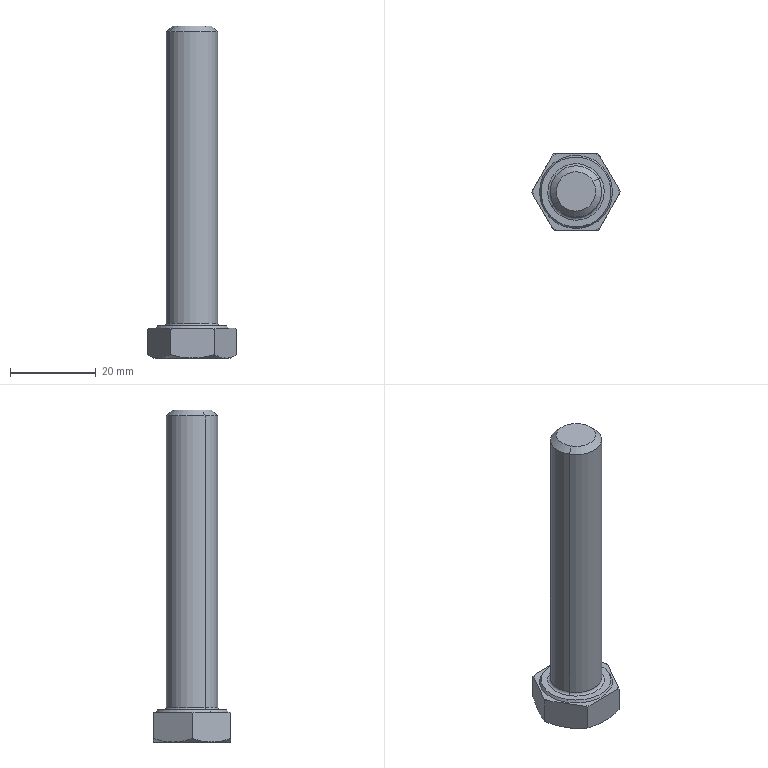Part | STEP file | BFACE2-29 | 1 solid | 30 faces | box 20.784 x 18.078 x 77.5 mm | volume 9947 mm3 | cone 16 | plane 10 | cylinder 2 | torus 2 | commonest cylinder face diameters 12 x2
STEP:
#1=CARTESIAN_POINT('',(-683.565,-263.234,3084.1));
#2=VERTEX_POINT('',#1);
#3=CARTESIAN_POINT('',(-693.912,-269.312,3084.1));
#4=VERTEX_POINT('',#3);
#5=CARTESIAN_POINT('',(-688.738,-266.273,3084.1));
#6=DIRECTION('',(0.,0.,-1.));
#7=DIRECTION('',(0.8622,0.5065,0.));
#8=AXIS2_PLACEMENT_3D('',#5,#6,#7);
#9=CIRCLE('',#8,6.);
#10=EDGE_CURVE('',#2,#4,#9,.T.);
#11=ORIENTED_EDGE('',*,*,#10,.F.);
#12=CARTESIAN_POINT('',(-683.565,-263.234,3152.1));
#13=VERTEX_POINT('',#12);
#14=CARTESIAN_POINT('',(-683.565,-263.234,3076.));
#15=DIRECTION('',(0.,0.,-1.));
#16=VECTOR('',#15,1000.);
#17=LINE('',#14,#16);
#18=EDGE_CURVE('',#13,#2,#17,.T.);
#19=ORIENTED_EDGE('',*,*,#18,.F.);
#20=CARTESIAN_POINT('',(-693.912,-269.312,3152.1));
#21=VERTEX_POINT('',#20);
#22=CARTESIAN_POINT('',(-688.738,-266.273,3152.1));
#23=DIRECTION('',(0.,0.,-1.));
#24=DIRECTION('',(-0.8622,-0.5065,0.));
#25=AXIS2_PLACEMENT_3D('',#22,#23,#24);
#26=CIRCLE('',#25,6.);
#27=EDGE_CURVE('',#13,#21,#26,.T.);
#28=ORIENTED_EDGE('',*,*,#27,.T.);
#29=CARTESIAN_POINT('',(-693.912,-269.312,3076.));
#30=DIRECTION('',(0.,0.,-1.));
#31=VECTOR('',#30,1000.);
#32=LINE('',#29,#31);
#33=EDGE_CURVE('',#21,#4,#32,.T.);
#34=ORIENTED_EDGE('',*,*,#33,.T.);
#35=EDGE_LOOP('',(#11,#19,#28,#34));
#36=FACE_OUTER_BOUND('',#35,.T.);
#37=CARTESIAN_POINT('',(-688.738,-266.273,3076.));
#38=DIRECTION('',(0.,0.,1.));
#39=DIRECTION('',(0.8622,0.5065,0.));
#40=AXIS2_PLACEMENT_3D('',#37,#38,#39);
#41=CYLINDRICAL_SURFACE('',#40,6.);
#42=ADVANCED_FACE('',(#36),#41,.T.);
#43=CARTESIAN_POINT('',(-692.705,-268.603,3153.5));
#44=VERTEX_POINT('',#43);
#45=CARTESIAN_POINT('',(-684.772,-263.943,3153.5));
#46=VERTEX_POINT('',#45);
#47=CARTESIAN_POINT('',(-688.738,-266.273,3153.5));
#48=DIRECTION('',(0.,0.,1.));
#49=DIRECTION('',(-0.8622,-0.5065,0.));
#50=AXIS2_PLACEMENT_3D('',#47,#48,#49);
#51=CIRCLE('',#50,4.6);
#52=EDGE_CURVE('',#44,#46,#51,.T.);
#53=ORIENTED_EDGE('',*,*,#52,.F.);
#54=CARTESIAN_POINT('',(-692.705,-268.603,3153.5));
#55=DIRECTION('',(-0.6097,-0.3582,-0.7071));
#56=VECTOR('',#55,1000.);
#57=LINE('',#54,#56);
#58=EDGE_CURVE('',#44,#21,#57,.T.);
#59=ORIENTED_EDGE('',*,*,#58,.T.);
#60=ORIENTED_EDGE('',*,*,#27,.F.);
#61=CARTESIAN_POINT('',(-684.772,-263.943,3153.5));
#62=DIRECTION('',(0.6097,0.3582,-0.7071));
#63=VECTOR('',#62,1000.);
#64=LINE('',#61,#63);
#65=EDGE_CURVE('',#46,#13,#64,.T.);
#66=ORIENTED_EDGE('',*,*,#65,.F.);
#67=EDGE_LOOP('',(#53,#59,#60,#66));
#68=FACE_OUTER_BOUND('',#67,.T.);
#69=CARTESIAN_POINT('',(-688.738,-266.273,3153.5));
#70=DIRECTION('',(0.,0.,-1.));
#71=DIRECTION('',(-0.8622,-0.5065,0.));
#72=AXIS2_PLACEMENT_3D('',#69,#70,#71);
#73=CONICAL_SURFACE('',#72,4.6,0.7854);
#74=ADVANCED_FACE('',(#68),#73,.T.);
#75=CARTESIAN_POINT('',(-694.429,-269.616,3083.5));
#76=VERTEX_POINT('',#75);
#77=CARTESIAN_POINT('',(-683.048,-262.93,3083.5));
#78=VERTEX_POINT('',#77);
#79=CARTESIAN_POINT('',(-688.738,-266.273,3083.5));
#80=DIRECTION('',(0.,0.,-1.));
#81=DIRECTION('',(0.8622,0.5065,0.));
#82=AXIS2_PLACEMENT_3D('',#79,#80,#81);
#83=CIRCLE('',#82,6.6);
#84=EDGE_CURVE('',#76,#78,#83,.T.);
#85=ORIENTED_EDGE('',*,*,#84,.F.);
#86=CARTESIAN_POINT('',(-694.429,-269.616,3084.1));
#87=DIRECTION('',(0.5065,-0.8622,0.));
#88=DIRECTION('',(0.8622,0.5065,0.));
#89=AXIS2_PLACEMENT_3D('',#86,#87,#88);
#90=CIRCLE('',#89,0.6);
#91=EDGE_CURVE('',#76,#4,#90,.T.);
#92=ORIENTED_EDGE('',*,*,#91,.T.);
#93=CARTESIAN_POINT('',(-688.738,-266.273,3084.1));
#94=DIRECTION('',(0.,0.,-1.));
#95=DIRECTION('',(0.8622,0.5065,0.));
#96=AXIS2_PLACEMENT_3D('',#93,#94,#95);
#97=CIRCLE('',#96,6.);
#98=EDGE_CURVE('',#4,#2,#97,.T.);
#99=ORIENTED_EDGE('',*,*,#98,.T.);
#100=CARTESIAN_POINT('',(-683.048,-262.93,3084.1));
#101=DIRECTION('',(-0.5065,0.8622,0.));
#102=DIRECTION('',(-0.8622,-0.5065,0.));
#103=AXIS2_PLACEMENT_3D('',#100,#101,#102);
#104=CIRCLE('',#103,0.6);
#105=EDGE_CURVE('',#78,#2,#104,.T.);
#106=ORIENTED_EDGE('',*,*,#105,.F.);
#107=EDGE_LOOP('',(#85,#92,#99,#106));
#108=FACE_OUTER_BOUND('',#107,.T.);
#109=CARTESIAN_POINT('',(-688.738,-266.273,3084.1));
#110=DIRECTION('',(0.,0.,-1.));
#111=DIRECTION('',(-0.8622,-0.5065,0.));
#112=AXIS2_PLACEMENT_3D('',#109,#110,#111);
#113=TOROIDAL_SURFACE('',#112,6.6,0.6);
#114=ADVANCED_FACE('',(#108),#113,.F.);
#115=CARTESIAN_POINT('',(-681.688,-262.131,3083.5));
#116=VERTEX_POINT('',#115);
#117=CARTESIAN_POINT('',(-695.789,-270.415,3083.5));
#118=VERTEX_POINT('',#117);
#119=CARTESIAN_POINT('',(-688.738,-266.273,3083.5));
#120=DIRECTION('',(0.,0.,-1.));
#121=DIRECTION('',(0.8622,0.5065,0.));
#122=AXIS2_PLACEMENT_3D('',#119,#120,#121);
#123=CIRCLE('',#122,8.177);
#124=EDGE_CURVE('',#116,#118,#123,.T.);
#125=ORIENTED_EDGE('',*,*,#124,.T.);
#126=CARTESIAN_POINT('',(-696.088,-270.59,3082.9));
#127=VERTEX_POINT('',#126);
#128=CARTESIAN_POINT('',(-696.088,-270.59,3082.9));
#129=DIRECTION('',(-0.4311,-0.2533,-0.866));
#130=VECTOR('',#129,1000.);
#131=LINE('',#128,#130);
#132=EDGE_CURVE('',#118,#127,#131,.T.);
#133=ORIENTED_EDGE('',*,*,#132,.T.);
#134=CARTESIAN_POINT('',(-681.389,-261.956,3082.9));
#135=VERTEX_POINT('',#134);
#136=CARTESIAN_POINT('',(-688.738,-266.273,3082.9));
#137=DIRECTION('',(0.,0.,-1.));
#138=DIRECTION('',(0.8622,0.5065,0.));
#139=AXIS2_PLACEMENT_3D('',#136,#137,#138);
#140=CIRCLE('',#139,8.524);
#141=EDGE_CURVE('',#135,#127,#140,.T.);
#142=ORIENTED_EDGE('',*,*,#141,.F.);
#143=CARTESIAN_POINT('',(-681.389,-261.956,3082.9));
#144=DIRECTION('',(0.4311,0.2533,-0.866));
#145=VECTOR('',#144,1000.);
#146=LINE('',#143,#145);
#147=EDGE_CURVE('',#116,#135,#146,.T.);
#148=ORIENTED_EDGE('',*,*,#147,.F.);
#149=EDGE_LOOP('',(#125,#133,#142,#148));
#150=FACE_OUTER_BOUND('',#149,.T.);
#151=CARTESIAN_POINT('',(-688.738,-266.273,3082.9));
#152=DIRECTION('',(0.,0.,-1.));
#153=DIRECTION('',(-0.8622,-0.5065,0.));
#154=AXIS2_PLACEMENT_3D('',#151,#152,#153);
#155=CONICAL_SURFACE('',#154,8.524,0.5236);
#156=ADVANCED_FACE('',(#150),#155,.T.);
#157=ORIENTED_EDGE('',*,*,#124,.F.);
#158=CARTESIAN_POINT('',(-688.738,-266.273,3083.5));
#159=DIRECTION('',(0.,0.,-1.));
#160=DIRECTION('',(0.8622,0.5065,0.));
#161=AXIS2_PLACEMENT_3D('',#158,#159,#160);
#162=CIRCLE('',#161,8.177);
#163=EDGE_CURVE('',#118,#116,#162,.T.);
#164=ORIENTED_EDGE('',*,*,#163,.F.);
#165=EDGE_LOOP('',(#157,#164));
#166=FACE_OUTER_BOUND('',#165,.T.);
#167=CARTESIAN_POINT('',(-688.738,-266.273,3083.5));
#168=DIRECTION('',(0.,0.,-1.));
#169=DIRECTION('',(0.8622,0.5065,0.));
#170=AXIS2_PLACEMENT_3D('',#167,#168,#169);
#171=CIRCLE('',#170,6.6);
#172=EDGE_CURVE('',#78,#76,#171,.T.);
#173=ORIENTED_EDGE('',*,*,#172,.T.);
#174=ORIENTED_EDGE('',*,*,#84,.T.);
#175=EDGE_LOOP('',(#173,#174));
#176=FACE_BOUND('',#175,.T.);
#177=CARTESIAN_POINT('',(-704.258,-275.39,3083.5));
#178=DIRECTION('',(0.,0.,1.));
#179=DIRECTION('',(0.8622,0.5065,0.));
#180=AXIS2_PLACEMENT_3D('',#177,#178,#179);
#181=PLANE('',#180);
#182=ADVANCED_FACE('',(#166,#176),#181,.T.);
#183=CARTESIAN_POINT('',(-693.118,-275.306,3082.9));
#184=VERTEX_POINT('',#183);
#185=CARTESIAN_POINT('',(-684.222,-275.239,3082.9));
#186=VERTEX_POINT('',#185);
#187=CARTESIAN_POINT('',(-693.866,-275.312,3082.9));
#188=DIRECTION('',(1.,0.007537,0.));
#189=VECTOR('',#188,1000.);
#190=LINE('',#187,#189);
#191=EDGE_CURVE('',#184,#186,#190,.T.);
#192=ORIENTED_EDGE('',*,*,#191,.F.);
#193=CARTESIAN_POINT('',(-693.866,-275.312,3082.696));
#194=VERTEX_POINT('',#193);
#195=CARTESIAN_POINT('',(-693.866,-275.312,3082.696));
#196=CARTESIAN_POINT('',(-693.618,-275.31,3082.768));
#197=CARTESIAN_POINT('',(-693.368,-275.308,3082.836));
#198=CARTESIAN_POINT('',(-693.118,-275.306,3082.9));
#199=B_SPLINE_CURVE_WITH_KNOTS('',3,(#195,#196,#197,#198),.UNSPECIFIED.,.F.,.F.,(4,4),(0.,1.),.UNSPECIFIED.);
#200=EDGE_CURVE('',#194,#184,#199,.T.);
#201=ORIENTED_EDGE('',*,*,#200,.F.);
#202=CARTESIAN_POINT('',(-693.866,-275.312,3076.804));
#203=VERTEX_POINT('',#202);
#204=CARTESIAN_POINT('',(-693.866,-275.312,3083.5));
#205=DIRECTION('',(0.,0.,-1.));
#206=VECTOR('',#205,1000.);
#207=LINE('',#204,#206);
#208=EDGE_CURVE('',#194,#203,#207,.T.);
#209=ORIENTED_EDGE('',*,*,#208,.T.);
#210=CARTESIAN_POINT('',(-688.67,-275.273,3076.));
#211=VERTEX_POINT('',#210);
#212=CARTESIAN_POINT('',(-688.67,-275.273,3076.));
#213=CARTESIAN_POINT('',(-689.557,-275.28,3076.));
#214=CARTESIAN_POINT('',(-690.432,-275.286,3076.077));
#215=CARTESIAN_POINT('',(-692.162,-275.299,3076.357));
#216=CARTESIAN_POINT('',(-693.018,-275.306,3076.559));
#217=CARTESIAN_POINT('',(-693.866,-275.312,3076.804));
#218=B_SPLINE_CURVE_WITH_KNOTS('',3,(#212,#213,#214,#215,#216,#217),.UNSPECIFIED.,.F.,.F.,(4,2,4),(0.,0.002629,0.005258),.UNSPECIFIED.);
#219=EDGE_CURVE('',#211,#203,#218,.T.);
#220=ORIENTED_EDGE('',*,*,#219,.F.);
#221=CARTESIAN_POINT('',(-683.474,-275.234,3076.804));
#222=VERTEX_POINT('',#221);
#223=CARTESIAN_POINT('',(-683.474,-275.234,3076.804));
#224=CARTESIAN_POINT('',(-684.323,-275.24,3076.559));
#225=CARTESIAN_POINT('',(-685.179,-275.247,3076.357));
#226=CARTESIAN_POINT('',(-686.909,-275.26,3076.077));
#227=CARTESIAN_POINT('',(-687.784,-275.266,3076.));
#228=CARTESIAN_POINT('',(-688.67,-275.273,3076.));
#229=B_SPLINE_CURVE_WITH_KNOTS('',3,(#223,#224,#225,#226,#227,#228),.UNSPECIFIED.,.F.,.F.,(4,2,4),(0.,0.002629,0.005258),.UNSPECIFIED.);
#230=EDGE_CURVE('',#222,#211,#229,.T.);
#231=ORIENTED_EDGE('',*,*,#230,.F.);
#232=CARTESIAN_POINT('',(-683.474,-275.234,3082.696));
#233=VERTEX_POINT('',#232);
#234=CARTESIAN_POINT('',(-683.474,-275.234,3083.5));
#235=DIRECTION('',(0.,0.,-1.));
#236=VECTOR('',#235,1000.);
#237=LINE('',#234,#236);
#238=EDGE_CURVE('',#233,#222,#237,.T.);
#239=ORIENTED_EDGE('',*,*,#238,.F.);
#240=CARTESIAN_POINT('',(-684.222,-275.239,3082.9));
#241=CARTESIAN_POINT('',(-683.972,-275.237,3082.836));
#242=CARTESIAN_POINT('',(-683.723,-275.236,3082.768));
#243=CARTESIAN_POINT('',(-683.474,-275.234,3082.696));
#244=B_SPLINE_CURVE_WITH_KNOTS('',3,(#240,#241,#242,#243),.UNSPECIFIED.,.F.,.F.,(4,4),(0.,1.),.UNSPECIFIED.);
#245=EDGE_CURVE('',#186,#233,#244,.T.);
#246=ORIENTED_EDGE('',*,*,#245,.F.);
#247=EDGE_LOOP('',(#192,#201,#209,#220,#231,#239,#246));
#248=FACE_OUTER_BOUND('',#247,.T.);
#249=CARTESIAN_POINT('',(-693.866,-275.312,3083.5));
#250=DIRECTION('',(-0.007537,1.,0.));
#251=DIRECTION('',(1.,0.007537,0.));
#252=AXIS2_PLACEMENT_3D('',#249,#250,#251);
#253=PLANE('',#252);
#254=ADVANCED_FACE('',(#248),#253,.F.);
#255=CARTESIAN_POINT('',(-683.105,-274.583,3082.9));
#256=VERTEX_POINT('',#255);
#257=CARTESIAN_POINT('',(-678.715,-266.845,3082.9));
#258=VERTEX_POINT('',#257);
#259=CARTESIAN_POINT('',(-683.474,-275.234,3082.9));
#260=DIRECTION('',(0.4935,0.8698,0.));
#261=VECTOR('',#260,1000.);
#262=LINE('',#259,#261);
#263=EDGE_CURVE('',#256,#258,#262,.T.);
#264=ORIENTED_EDGE('',*,*,#263,.F.);
#265=CARTESIAN_POINT('',(-683.474,-275.234,3082.696));
#266=CARTESIAN_POINT('',(-683.352,-275.017,3082.768));
#267=CARTESIAN_POINT('',(-683.229,-274.8,3082.836));
#268=CARTESIAN_POINT('',(-683.105,-274.583,3082.9));
#269=B_SPLINE_CURVE_WITH_KNOTS('',3,(#265,#266,#267,#268),.UNSPECIFIED.,.F.,.F.,(4,4),(0.,1.),.UNSPECIFIED.);
#270=EDGE_CURVE('',#233,#256,#269,.T.);
#271=ORIENTED_EDGE('',*,*,#270,.F.);
#272=ORIENTED_EDGE('',*,*,#238,.T.);
#273=CARTESIAN_POINT('',(-680.91,-270.714,3076.));
#274=VERTEX_POINT('',#273);
#275=CARTESIAN_POINT('',(-680.91,-270.714,3076.));
#276=CARTESIAN_POINT('',(-681.348,-271.486,3076.));
#277=CARTESIAN_POINT('',(-681.78,-272.246,3076.077));
#278=CARTESIAN_POINT('',(-682.633,-273.751,3076.357));
#279=CARTESIAN_POINT('',(-683.056,-274.495,3076.559));
#280=CARTESIAN_POINT('',(-683.474,-275.234,3076.804));
#281=B_SPLINE_CURVE_WITH_KNOTS('',3,(#275,#276,#277,#278,#279,#280),.UNSPECIFIED.,.F.,.F.,(4,2,4),(0.,0.002629,0.005258),.UNSPECIFIED.);
#282=EDGE_CURVE('',#274,#222,#281,.T.);
#283=ORIENTED_EDGE('',*,*,#282,.F.);
#284=CARTESIAN_POINT('',(-678.346,-266.195,3076.804));
#285=VERTEX_POINT('',#284);
#286=CARTESIAN_POINT('',(-678.346,-266.195,3076.804));
#287=CARTESIAN_POINT('',(-678.765,-266.933,3076.559));
#288=CARTESIAN_POINT('',(-679.187,-267.677,3076.357));
#289=CARTESIAN_POINT('',(-680.041,-269.182,3076.077));
#290=CARTESIAN_POINT('',(-680.473,-269.943,3076.));
#291=CARTESIAN_POINT('',(-680.91,-270.714,3076.));
#292=B_SPLINE_CURVE_WITH_KNOTS('',3,(#286,#287,#288,#289,#290,#291),.UNSPECIFIED.,.F.,.F.,(4,2,4),(0.,0.002629,0.005258),.UNSPECIFIED.);
#293=EDGE_CURVE('',#285,#274,#292,.T.);
#294=ORIENTED_EDGE('',*,*,#293,.F.);
#295=CARTESIAN_POINT('',(-678.346,-266.195,3082.696));
#296=VERTEX_POINT('',#295);
#297=CARTESIAN_POINT('',(-678.346,-266.195,3083.5));
#298=DIRECTION('',(0.,0.,-1.));
#299=VECTOR('',#298,1000.);
#300=LINE('',#297,#299);
#301=EDGE_CURVE('',#296,#285,#300,.T.);
#302=ORIENTED_EDGE('',*,*,#301,.F.);
#303=CARTESIAN_POINT('',(-678.715,-266.845,3082.9));
#304=CARTESIAN_POINT('',(-678.592,-266.628,3082.836));
#305=CARTESIAN_POINT('',(-678.469,-266.411,3082.768));
#306=CARTESIAN_POINT('',(-678.346,-266.195,3082.696));
#307=B_SPLINE_CURVE_WITH_KNOTS('',3,(#303,#304,#305,#306),.UNSPECIFIED.,.F.,.F.,(4,4),(0.,1.),.UNSPECIFIED.);
#308=EDGE_CURVE('',#258,#296,#307,.T.);
#309=ORIENTED_EDGE('',*,*,#308,.F.);
#310=EDGE_LOOP('',(#264,#271,#272,#283,#294,#302,#309));
#311=FACE_OUTER_BOUND('',#310,.T.);
#312=CARTESIAN_POINT('',(-683.474,-275.234,3083.5));
#313=DIRECTION('',(-0.8698,0.4935,0.));
#314=DIRECTION('',(0.4935,0.8698,0.));
#315=AXIS2_PLACEMENT_3D('',#312,#313,#314);
#316=PLANE('',#315);
#317=ADVANCED_FACE('',(#311),#316,.F.);
#318=CARTESIAN_POINT('',(-678.725,-265.55,3082.9));
#319=VERTEX_POINT('',#318);
#320=CARTESIAN_POINT('',(-683.231,-257.879,3082.9));
#321=VERTEX_POINT('',#320);
#322=CARTESIAN_POINT('',(-678.346,-266.195,3082.9));
#323=DIRECTION('',(-0.5065,0.8622,0.));
#324=VECTOR('',#323,1000.);
#325=LINE('',#322,#324);
#326=EDGE_CURVE('',#319,#321,#325,.T.);
#327=ORIENTED_EDGE('',*,*,#326,.F.);
#328=CARTESIAN_POINT('',(-678.346,-266.195,3082.696));
#329=CARTESIAN_POINT('',(-678.472,-265.981,3082.768));
#330=CARTESIAN_POINT('',(-678.598,-265.766,3082.836));
#331=CARTESIAN_POINT('',(-678.725,-265.55,3082.9));
#332=B_SPLINE_CURVE_WITH_KNOTS('',3,(#328,#329,#330,#331),.UNSPECIFIED.,.F.,.F.,(4,4),(0.,1.),.UNSPECIFIED.);
#333=EDGE_CURVE('',#296,#319,#332,.T.);
#334=ORIENTED_EDGE('',*,*,#333,.F.);
#335=ORIENTED_EDGE('',*,*,#301,.T.);
#336=CARTESIAN_POINT('',(-680.978,-261.715,3076.));
#337=VERTEX_POINT('',#336);
#338=CARTESIAN_POINT('',(-680.978,-261.715,3076.));
#339=CARTESIAN_POINT('',(-680.529,-262.479,3076.));
#340=CARTESIAN_POINT('',(-680.086,-263.233,3076.077));
#341=CARTESIAN_POINT('',(-679.21,-264.725,3076.357));
#342=CARTESIAN_POINT('',(-678.776,-265.463,3076.559));
#343=CARTESIAN_POINT('',(-678.346,-266.195,3076.804));
#344=B_SPLINE_CURVE_WITH_KNOTS('',3,(#338,#339,#340,#341,#342,#343),.UNSPECIFIED.,.F.,.F.,(4,2,4),(0.,0.002629,0.005258),.UNSPECIFIED.);
#345=EDGE_CURVE('',#337,#285,#344,.T.);
#346=ORIENTED_EDGE('',*,*,#345,.F.);
#347=CARTESIAN_POINT('',(-683.61,-257.234,3076.804));
#348=VERTEX_POINT('',#347);
#349=CARTESIAN_POINT('',(-683.61,-257.234,3076.804));
#350=CARTESIAN_POINT('',(-683.18,-257.966,3076.559));
#351=CARTESIAN_POINT('',(-682.747,-258.704,3076.357));
#352=CARTESIAN_POINT('',(-681.87,-260.196,3076.077));
#353=CARTESIAN_POINT('',(-681.427,-260.95,3076.));
#354=CARTESIAN_POINT('',(-680.978,-261.715,3076.));
#355=B_SPLINE_CURVE_WITH_KNOTS('',3,(#349,#350,#351,#352,#353,#354),.UNSPECIFIED.,.F.,.F.,(4,2,4),(0.,0.002629,0.005258),.UNSPECIFIED.);
#356=EDGE_CURVE('',#348,#337,#355,.T.);
#357=ORIENTED_EDGE('',*,*,#356,.F.);
#358=CARTESIAN_POINT('',(-683.61,-257.234,3082.696));
#359=VERTEX_POINT('',#358);
#360=CARTESIAN_POINT('',(-683.61,-257.234,3083.5));
#361=DIRECTION('',(0.,0.,-1.));
#362=VECTOR('',#361,1000.);
#363=LINE('',#360,#362);
#364=EDGE_CURVE('',#359,#348,#363,.T.);
#365=ORIENTED_EDGE('',*,*,#364,.F.);
#366=CARTESIAN_POINT('',(-683.231,-257.879,3082.9));
#367=CARTESIAN_POINT('',(-683.358,-257.663,3082.836));
#368=CARTESIAN_POINT('',(-683.485,-257.448,3082.768));
#369=CARTESIAN_POINT('',(-683.61,-257.234,3082.696));
#370=B_SPLINE_CURVE_WITH_KNOTS('',3,(#366,#367,#368,#369),.UNSPECIFIED.,.F.,.F.,(4,4),(0.,1.),.UNSPECIFIED.);
#371=EDGE_CURVE('',#321,#359,#370,.T.);
#372=ORIENTED_EDGE('',*,*,#371,.F.);
#373=EDGE_LOOP('',(#327,#334,#335,#346,#357,#365,#372));
#374=FACE_OUTER_BOUND('',#373,.T.);
#375=CARTESIAN_POINT('',(-678.346,-266.195,3083.5));
#376=DIRECTION('',(-0.8622,-0.5065,0.));
#377=DIRECTION('',(-0.5065,0.8622,0.));
#378=AXIS2_PLACEMENT_3D('',#375,#376,#377);
#379=PLANE('',#378);
#380=ADVANCED_FACE('',(#374),#379,.F.);
#381=CARTESIAN_POINT('',(-684.358,-257.24,3082.9));
#382=VERTEX_POINT('',#381);
#383=CARTESIAN_POINT('',(-693.254,-257.307,3082.9));
#384=VERTEX_POINT('',#383);
#385=CARTESIAN_POINT('',(-694.002,-257.313,3082.9));
#386=DIRECTION('',(-1.,-0.007537,0.));
#387=VECTOR('',#386,1000.);
#388=LINE('',#385,#387);
#389=EDGE_CURVE('',#382,#384,#388,.T.);
#390=ORIENTED_EDGE('',*,*,#389,.F.);
#391=CARTESIAN_POINT('',(-683.61,-257.234,3082.696));
#392=CARTESIAN_POINT('',(-683.859,-257.236,3082.768));
#393=CARTESIAN_POINT('',(-684.108,-257.238,3082.836));
#394=CARTESIAN_POINT('',(-684.358,-257.24,3082.9));
#395=B_SPLINE_CURVE_WITH_KNOTS('',3,(#391,#392,#393,#394),.UNSPECIFIED.,.F.,.F.,(4,4),(0.,1.),.UNSPECIFIED.);
#396=EDGE_CURVE('',#359,#382,#395,.T.);
#397=ORIENTED_EDGE('',*,*,#396,.F.);
#398=ORIENTED_EDGE('',*,*,#364,.T.);
#399=CARTESIAN_POINT('',(-688.806,-257.273,3076.));
#400=VERTEX_POINT('',#399);
#401=CARTESIAN_POINT('',(-688.806,-257.273,3076.));
#402=CARTESIAN_POINT('',(-687.919,-257.267,3076.));
#403=CARTESIAN_POINT('',(-687.045,-257.26,3076.077));
#404=CARTESIAN_POINT('',(-685.314,-257.247,3076.357));
#405=CARTESIAN_POINT('',(-684.459,-257.241,3076.559));
#406=CARTESIAN_POINT('',(-683.61,-257.234,3076.804));
#407=B_SPLINE_CURVE_WITH_KNOTS('',3,(#401,#402,#403,#404,#405,#406),.UNSPECIFIED.,.F.,.F.,(4,2,4),(0.,0.002629,0.005258),.UNSPECIFIED.);
#408=EDGE_CURVE('',#400,#348,#407,.T.);
#409=ORIENTED_EDGE('',*,*,#408,.F.);
#410=CARTESIAN_POINT('',(-694.002,-257.313,3076.804));
#411=VERTEX_POINT('',#410);
#412=CARTESIAN_POINT('',(-694.002,-257.313,3076.804));
#413=CARTESIAN_POINT('',(-693.153,-257.306,3076.559));
#414=CARTESIAN_POINT('',(-692.298,-257.3,3076.357));
#415=CARTESIAN_POINT('',(-690.568,-257.287,3076.077));
#416=CARTESIAN_POINT('',(-689.693,-257.28,3076.));
#417=CARTESIAN_POINT('',(-688.806,-257.273,3076.));
#418=B_SPLINE_CURVE_WITH_KNOTS('',3,(#412,#413,#414,#415,#416,#417),.UNSPECIFIED.,.F.,.F.,(4,2,4),(0.,0.002629,0.005258),.UNSPECIFIED.);
#419=EDGE_CURVE('',#411,#400,#418,.T.);
#420=ORIENTED_EDGE('',*,*,#419,.F.);
#421=CARTESIAN_POINT('',(-694.002,-257.313,3082.696));
#422=VERTEX_POINT('',#421);
#423=CARTESIAN_POINT('',(-694.002,-257.313,3083.5));
#424=DIRECTION('',(0.,0.,-1.));
#425=VECTOR('',#424,1000.);
#426=LINE('',#423,#425);
#427=EDGE_CURVE('',#422,#411,#426,.T.);
#428=ORIENTED_EDGE('',*,*,#427,.F.);
#429=CARTESIAN_POINT('',(-693.254,-257.307,3082.9));
#430=CARTESIAN_POINT('',(-693.504,-257.309,3082.836));
#431=CARTESIAN_POINT('',(-693.753,-257.311,3082.768));
#432=CARTESIAN_POINT('',(-694.002,-257.313,3082.696));
#433=B_SPLINE_CURVE_WITH_KNOTS('',3,(#429,#430,#431,#432),.UNSPECIFIED.,.F.,.F.,(4,4),(0.,1.),.UNSPECIFIED.);
#434=EDGE_CURVE('',#384,#422,#433,.T.);
#435=ORIENTED_EDGE('',*,*,#434,.F.);
#436=EDGE_LOOP('',(#390,#397,#398,#409,#420,#428,#435));
#437=FACE_OUTER_BOUND('',#436,.T.);
#438=CARTESIAN_POINT('',(-694.002,-257.313,3083.5));
#439=DIRECTION('',(0.007537,-1.,0.));
#440=DIRECTION('',(-1.,-0.007537,0.));
#441=AXIS2_PLACEMENT_3D('',#438,#439,#440);
#442=PLANE('',#441);
#443=ADVANCED_FACE('',(#437),#442,.F.);
#444=CARTESIAN_POINT('',(-694.371,-257.963,3082.9));
#445=VERTEX_POINT('',#444);
#446=CARTESIAN_POINT('',(-698.761,-265.701,3082.9));
#447=VERTEX_POINT('',#446);
#448=CARTESIAN_POINT('',(-699.13,-266.351,3082.9));
#449=DIRECTION('',(-0.4935,-0.8698,0.));
#450=VECTOR('',#449,1000.);
#451=LINE('',#448,#450);
#452=EDGE_CURVE('',#445,#447,#451,.T.);
#453=ORIENTED_EDGE('',*,*,#452,.F.);
#454=CARTESIAN_POINT('',(-694.002,-257.313,3082.696));
#455=CARTESIAN_POINT('',(-694.125,-257.529,3082.768));
#456=CARTESIAN_POINT('',(-694.248,-257.746,3082.836));
#457=CARTESIAN_POINT('',(-694.371,-257.963,3082.9));
#458=B_SPLINE_CURVE_WITH_KNOTS('',3,(#454,#455,#456,#457),.UNSPECIFIED.,.F.,.F.,(4,4),(0.,1.),.UNSPECIFIED.);
#459=EDGE_CURVE('',#422,#445,#458,.T.);
#460=ORIENTED_EDGE('',*,*,#459,.F.);
#461=ORIENTED_EDGE('',*,*,#427,.T.);
#462=CARTESIAN_POINT('',(-696.566,-261.832,3076.));
#463=VERTEX_POINT('',#462);
#464=CARTESIAN_POINT('',(-696.566,-261.832,3076.));
#465=CARTESIAN_POINT('',(-696.129,-261.061,3076.));
#466=CARTESIAN_POINT('',(-695.697,-260.3,3076.077));
#467=CARTESIAN_POINT('',(-694.843,-258.795,3076.357));
#468=CARTESIAN_POINT('',(-694.421,-258.051,3076.559));
#469=CARTESIAN_POINT('',(-694.002,-257.313,3076.804));
#470=B_SPLINE_CURVE_WITH_KNOTS('',3,(#464,#465,#466,#467,#468,#469),.UNSPECIFIED.,.F.,.F.,(4,2,4),(0.,0.002629,0.005258),.UNSPECIFIED.);
#471=EDGE_CURVE('',#463,#411,#470,.T.);
#472=ORIENTED_EDGE('',*,*,#471,.F.);
#473=CARTESIAN_POINT('',(-699.13,-266.351,3076.804));
#474=VERTEX_POINT('',#473);
#475=CARTESIAN_POINT('',(-699.13,-266.351,3076.804));
#476=CARTESIAN_POINT('',(-698.711,-265.613,3076.559));
#477=CARTESIAN_POINT('',(-698.289,-264.869,3076.357));
#478=CARTESIAN_POINT('',(-697.435,-263.364,3076.077));
#479=CARTESIAN_POINT('',(-697.004,-262.603,3076.));
#480=CARTESIAN_POINT('',(-696.566,-261.832,3076.));
#481=B_SPLINE_CURVE_WITH_KNOTS('',3,(#475,#476,#477,#478,#479,#480),.UNSPECIFIED.,.F.,.F.,(4,2,4),(0.,0.002629,0.005258),.UNSPECIFIED.);
#482=EDGE_CURVE('',#474,#463,#481,.T.);
#483=ORIENTED_EDGE('',*,*,#482,.F.);
#484=CARTESIAN_POINT('',(-699.13,-266.351,3082.696));
#485=VERTEX_POINT('',#484);
#486=CARTESIAN_POINT('',(-699.13,-266.351,3083.5));
#487=DIRECTION('',(0.,0.,-1.));
#488=VECTOR('',#487,1000.);
#489=LINE('',#486,#488);
#490=EDGE_CURVE('',#485,#474,#489,.T.);
#491=ORIENTED_EDGE('',*,*,#490,.F.);
#492=CARTESIAN_POINT('',(-698.761,-265.701,3082.9));
#493=CARTESIAN_POINT('',(-698.885,-265.918,3082.836));
#494=CARTESIAN_POINT('',(-699.008,-266.135,3082.768));
#495=CARTESIAN_POINT('',(-699.13,-266.351,3082.696));
#496=B_SPLINE_CURVE_WITH_KNOTS('',3,(#492,#493,#494,#495),.UNSPECIFIED.,.F.,.F.,(4,4),(0.,1.),.UNSPECIFIED.);
#497=EDGE_CURVE('',#447,#485,#496,.T.);
#498=ORIENTED_EDGE('',*,*,#497,.F.);
#499=EDGE_LOOP('',(#453,#460,#461,#472,#483,#491,#498));
#500=FACE_OUTER_BOUND('',#499,.T.);
#501=CARTESIAN_POINT('',(-699.13,-266.351,3083.5));
#502=DIRECTION('',(0.8698,-0.4935,0.));
#503=DIRECTION('',(-0.4935,-0.8698,0.));
#504=AXIS2_PLACEMENT_3D('',#501,#502,#503);
#505=PLANE('',#504);
#506=ADVANCED_FACE('',(#500),#505,.F.);
#507=CARTESIAN_POINT('',(-698.751,-266.996,3082.9));
#508=VERTEX_POINT('',#507);
#509=CARTESIAN_POINT('',(-694.245,-274.667,3082.9));
#510=VERTEX_POINT('',#509);
#511=CARTESIAN_POINT('',(-693.866,-275.312,3082.9));
#512=DIRECTION('',(0.5065,-0.8622,0.));
#513=VECTOR('',#512,1000.);
#514=LINE('',#511,#513);
#515=EDGE_CURVE('',#508,#510,#514,.T.);
#516=ORIENTED_EDGE('',*,*,#515,.F.);
#517=CARTESIAN_POINT('',(-699.13,-266.351,3082.696));
#518=CARTESIAN_POINT('',(-699.005,-266.565,3082.768));
#519=CARTESIAN_POINT('',(-698.878,-266.78,3082.836));
#520=CARTESIAN_POINT('',(-698.751,-266.996,3082.9));
#521=B_SPLINE_CURVE_WITH_KNOTS('',3,(#517,#518,#519,#520),.UNSPECIFIED.,.F.,.F.,(4,4),(0.,1.),.UNSPECIFIED.);
#522=EDGE_CURVE('',#485,#508,#521,.T.);
#523=ORIENTED_EDGE('',*,*,#522,.F.);
#524=ORIENTED_EDGE('',*,*,#490,.T.);
#525=CARTESIAN_POINT('',(-696.498,-270.832,3076.));
#526=VERTEX_POINT('',#525);
#527=CARTESIAN_POINT('',(-696.498,-270.832,3076.));
#528=CARTESIAN_POINT('',(-696.948,-270.067,3076.));
#529=CARTESIAN_POINT('',(-697.391,-269.313,3076.077));
#530=CARTESIAN_POINT('',(-698.267,-267.821,3076.357));
#531=CARTESIAN_POINT('',(-698.7,-267.083,3076.559));
#532=CARTESIAN_POINT('',(-699.13,-266.351,3076.804));
#533=B_SPLINE_CURVE_WITH_KNOTS('',3,(#527,#528,#529,#530,#531,#532),.UNSPECIFIED.,.F.,.F.,(4,2,4),(0.,0.002629,0.005258),.UNSPECIFIED.);
#534=EDGE_CURVE('',#526,#474,#533,.T.);
#535=ORIENTED_EDGE('',*,*,#534,.F.);
#536=CARTESIAN_POINT('',(-693.866,-275.312,3076.804));
#537=CARTESIAN_POINT('',(-694.296,-274.58,3076.559));
#538=CARTESIAN_POINT('',(-694.73,-273.843,3076.357));
#539=CARTESIAN_POINT('',(-695.606,-272.351,3076.077));
#540=CARTESIAN_POINT('',(-696.049,-271.596,3076.));
#541=CARTESIAN_POINT('',(-696.498,-270.832,3076.));
#542=B_SPLINE_CURVE_WITH_KNOTS('',3,(#536,#537,#538,#539,#540,#541),.UNSPECIFIED.,.F.,.F.,(4,2,4),(0.,0.002629,0.005258),.UNSPECIFIED.);
#543=EDGE_CURVE('',#203,#526,#542,.T.);
#544=ORIENTED_EDGE('',*,*,#543,.F.);
#545=ORIENTED_EDGE('',*,*,#208,.F.);
#546=CARTESIAN_POINT('',(-694.245,-274.667,3082.9));
#547=CARTESIAN_POINT('',(-694.119,-274.883,3082.836));
#548=CARTESIAN_POINT('',(-693.992,-275.098,3082.768));
#549=CARTESIAN_POINT('',(-693.866,-275.312,3082.696));
#550=B_SPLINE_CURVE_WITH_KNOTS('',3,(#546,#547,#548,#549),.UNSPECIFIED.,.F.,.F.,(4,4),(0.,1.),.UNSPECIFIED.);
#551=EDGE_CURVE('',#510,#194,#550,.T.);
#552=ORIENTED_EDGE('',*,*,#551,.F.);
#553=EDGE_LOOP('',(#516,#523,#524,#535,#544,#545,#552));
#554=FACE_OUTER_BOUND('',#553,.T.);
#555=CARTESIAN_POINT('',(-693.866,-275.312,3083.5));
#556=DIRECTION('',(0.8622,0.5065,0.));
#557=DIRECTION('',(0.5065,-0.8622,0.));
#558=AXIS2_PLACEMENT_3D('',#555,#556,#557);
#559=PLANE('',#558);
#560=ADVANCED_FACE('',(#554),#559,.F.);
#561=ORIENTED_EDGE('',*,*,#522,.T.);
#562=CARTESIAN_POINT('',(-688.738,-266.273,3082.9));
#563=DIRECTION('',(0.,0.,-1.));
#564=DIRECTION('',(-0.8622,-0.5065,0.));
#565=AXIS2_PLACEMENT_3D('',#562,#563,#564);
#566=CIRCLE('',#565,10.039);
#567=EDGE_CURVE('',#508,#447,#566,.T.);
#568=ORIENTED_EDGE('',*,*,#567,.T.);
#569=ORIENTED_EDGE('',*,*,#497,.T.);
#570=EDGE_LOOP('',(#561,#568,#569));
#571=FACE_OUTER_BOUND('',#570,.T.);
#572=CARTESIAN_POINT('',(-688.738,-266.273,3079.809));
#573=DIRECTION('',(0.,0.,-1.));
#574=DIRECTION('',(-0.8622,-0.5065,0.));
#575=AXIS2_PLACEMENT_3D('',#572,#573,#574);
#576=CONICAL_SURFACE('',#575,15.392,1.047);
#577=ADVANCED_FACE('',(#571),#576,.T.);
#578=ORIENTED_EDGE('',*,*,#459,.T.);
#579=CARTESIAN_POINT('',(-688.738,-266.273,3082.9));
#580=DIRECTION('',(0.,0.,-1.));
#581=DIRECTION('',(-0.8622,-0.5065,0.));
#582=AXIS2_PLACEMENT_3D('',#579,#580,#581);
#583=CIRCLE('',#582,10.039);
#584=EDGE_CURVE('',#445,#384,#583,.T.);
#585=ORIENTED_EDGE('',*,*,#584,.T.);
#586=ORIENTED_EDGE('',*,*,#434,.T.);
#587=EDGE_LOOP('',(#578,#585,#586));
#588=FACE_OUTER_BOUND('',#587,.T.);
#589=CARTESIAN_POINT('',(-688.738,-266.273,3079.809));
#590=DIRECTION('',(0.,0.,-1.));
#591=DIRECTION('',(-0.8622,-0.5065,0.));
#592=AXIS2_PLACEMENT_3D('',#589,#590,#591);
#593=CONICAL_SURFACE('',#592,15.392,1.047);
#594=ADVANCED_FACE('',(#588),#593,.T.);
#595=ORIENTED_EDGE('',*,*,#396,.T.);
#596=CARTESIAN_POINT('',(-688.738,-266.273,3082.9));
#597=DIRECTION('',(0.,0.,-1.));
#598=DIRECTION('',(-0.8622,-0.5065,0.));
#599=AXIS2_PLACEMENT_3D('',#596,#597,#598);
#600=CIRCLE('',#599,10.039);
#601=EDGE_CURVE('',#382,#321,#600,.T.);
#602=ORIENTED_EDGE('',*,*,#601,.T.);
#603=ORIENTED_EDGE('',*,*,#371,.T.);
#604=EDGE_LOOP('',(#595,#602,#603));
#605=FACE_OUTER_BOUND('',#604,.T.);
#606=CARTESIAN_POINT('',(-688.738,-266.273,3079.809));
#607=DIRECTION('',(0.,0.,-1.));
#608=DIRECTION('',(-0.8622,-0.5065,0.));
#609=AXIS2_PLACEMENT_3D('',#606,#607,#608);
#610=CONICAL_SURFACE('',#609,15.392,1.047);
#611=ADVANCED_FACE('',(#605),#610,.T.);
#612=ORIENTED_EDGE('',*,*,#333,.T.);
#613=CARTESIAN_POINT('',(-688.738,-266.273,3082.9));
#614=DIRECTION('',(0.,0.,-1.));
#615=DIRECTION('',(-0.8622,-0.5065,0.));
#616=AXIS2_PLACEMENT_3D('',#613,#614,#615);
#617=CIRCLE('',#616,10.039);
#618=EDGE_CURVE('',#319,#258,#617,.T.);
#619=ORIENTED_EDGE('',*,*,#618,.T.);
#620=ORIENTED_EDGE('',*,*,#308,.T.);
#621=EDGE_LOOP('',(#612,#619,#620));
#622=FACE_OUTER_BOUND('',#621,.T.);
#623=CARTESIAN_POINT('',(-688.738,-266.273,3079.809));
#624=DIRECTION('',(0.,0.,-1.));
#625=DIRECTION('',(-0.8622,-0.5065,0.));
#626=AXIS2_PLACEMENT_3D('',#623,#624,#625);
#627=CONICAL_SURFACE('',#626,15.392,1.047);
#628=ADVANCED_FACE('',(#622),#627,.T.);
#629=ORIENTED_EDGE('',*,*,#270,.T.);
#630=CARTESIAN_POINT('',(-688.738,-266.273,3082.9));
#631=DIRECTION('',(0.,0.,-1.));
#632=DIRECTION('',(-0.8622,-0.5065,0.));
#633=AXIS2_PLACEMENT_3D('',#630,#631,#632);
#634=CIRCLE('',#633,10.039);
#635=EDGE_CURVE('',#256,#186,#634,.T.);
#636=ORIENTED_EDGE('',*,*,#635,.T.);
#637=ORIENTED_EDGE('',*,*,#245,.T.);
#638=EDGE_LOOP('',(#629,#636,#637));
#639=FACE_OUTER_BOUND('',#638,.T.);
#640=CARTESIAN_POINT('',(-688.738,-266.273,3079.809));
#641=DIRECTION('',(0.,0.,-1.));
#642=DIRECTION('',(-0.8622,-0.5065,0.));
#643=AXIS2_PLACEMENT_3D('',#640,#641,#642);
#644=CONICAL_SURFACE('',#643,15.392,1.047);
#645=ADVANCED_FACE('',(#639),#644,.T.);
#646=ORIENTED_EDGE('',*,*,#200,.T.);
#647=CARTESIAN_POINT('',(-688.738,-266.273,3082.9));
#648=DIRECTION('',(0.,0.,-1.));
#649=DIRECTION('',(-0.8622,-0.5065,0.));
#650=AXIS2_PLACEMENT_3D('',#647,#648,#649);
#651=CIRCLE('',#650,10.039);
#652=EDGE_CURVE('',#184,#510,#651,.T.);
#653=ORIENTED_EDGE('',*,*,#652,.T.);
#654=ORIENTED_EDGE('',*,*,#551,.T.);
#655=EDGE_LOOP('',(#646,#653,#654));
#656=FACE_OUTER_BOUND('',#655,.T.);
#657=CARTESIAN_POINT('',(-688.738,-266.273,3079.809));
#658=DIRECTION('',(0.,0.,-1.));
#659=DIRECTION('',(-0.8622,-0.5065,0.));
#660=AXIS2_PLACEMENT_3D('',#657,#658,#659);
#661=CONICAL_SURFACE('',#660,15.392,1.047);
#662=ADVANCED_FACE('',(#656),#661,.T.);
#663=ORIENTED_EDGE('',*,*,#482,.T.);
#664=CARTESIAN_POINT('',(-688.738,-266.273,3076.));
#665=DIRECTION('',(0.,0.,1.));
#666=DIRECTION('',(-0.8622,-0.5065,0.));
#667=AXIS2_PLACEMENT_3D('',#664,#665,#666);
#668=CIRCLE('',#667,9.);
#669=EDGE_CURVE('',#463,#526,#668,.T.);
#670=ORIENTED_EDGE('',*,*,#669,.T.);
#671=ORIENTED_EDGE('',*,*,#534,.T.);
#672=EDGE_LOOP('',(#663,#670,#671));
#673=FACE_OUTER_BOUND('',#672,.T.);
#674=CARTESIAN_POINT('',(-688.738,-266.273,3076.));
#675=DIRECTION('',(0.,0.,1.));
#676=DIRECTION('',(0.8622,0.5065,0.));
#677=AXIS2_PLACEMENT_3D('',#674,#675,#676);
#678=CONICAL_SURFACE('',#677,9.,1.047);
#679=ADVANCED_FACE('',(#673),#678,.T.);
#680=ORIENTED_EDGE('',*,*,#419,.T.);
#681=CARTESIAN_POINT('',(-688.738,-266.273,3076.));
#682=DIRECTION('',(0.,0.,1.));
#683=DIRECTION('',(-0.8622,-0.5065,0.));
#684=AXIS2_PLACEMENT_3D('',#681,#682,#683);
#685=CIRCLE('',#684,9.);
#686=EDGE_CURVE('',#400,#463,#685,.T.);
#687=ORIENTED_EDGE('',*,*,#686,.T.);
#688=ORIENTED_EDGE('',*,*,#471,.T.);
#689=EDGE_LOOP('',(#680,#687,#688));
#690=FACE_OUTER_BOUND('',#689,.T.);
#691=CARTESIAN_POINT('',(-688.738,-266.273,3076.));
#692=DIRECTION('',(0.,0.,1.));
#693=DIRECTION('',(0.8622,0.5065,0.));
#694=AXIS2_PLACEMENT_3D('',#691,#692,#693);
#695=CONICAL_SURFACE('',#694,9.,1.047);
#696=ADVANCED_FACE('',(#690),#695,.T.);
#697=ORIENTED_EDGE('',*,*,#356,.T.);
#698=CARTESIAN_POINT('',(-688.738,-266.273,3076.));
#699=DIRECTION('',(0.,0.,1.));
#700=DIRECTION('',(-0.8622,-0.5065,0.));
#701=AXIS2_PLACEMENT_3D('',#698,#699,#700);
#702=CIRCLE('',#701,9.);
#703=EDGE_CURVE('',#337,#400,#702,.T.);
#704=ORIENTED_EDGE('',*,*,#703,.T.);
#705=ORIENTED_EDGE('',*,*,#408,.T.);
#706=EDGE_LOOP('',(#697,#704,#705));
#707=FACE_OUTER_BOUND('',#706,.T.);
#708=CARTESIAN_POINT('',(-688.738,-266.273,3076.));
#709=DIRECTION('',(0.,0.,1.));
#710=DIRECTION('',(0.8622,0.5065,0.));
#711=AXIS2_PLACEMENT_3D('',#708,#709,#710);
#712=CONICAL_SURFACE('',#711,9.,1.047);
#713=ADVANCED_FACE('',(#707),#712,.T.);
#714=ORIENTED_EDGE('',*,*,#345,.T.);
#715=ORIENTED_EDGE('',*,*,#293,.T.);
#716=CARTESIAN_POINT('',(-688.738,-266.273,3076.));
#717=DIRECTION('',(0.,0.,-1.));
#718=DIRECTION('',(0.8622,0.5065,0.));
#719=AXIS2_PLACEMENT_3D('',#716,#717,#718);
#720=CIRCLE('',#719,9.);
#721=EDGE_CURVE('',#337,#274,#720,.T.);
#722=ORIENTED_EDGE('',*,*,#721,.F.);
#723=EDGE_LOOP('',(#714,#715,#722));
#724=FACE_OUTER_BOUND('',#723,.T.);
#725=CARTESIAN_POINT('',(-688.738,-266.273,3076.));
#726=DIRECTION('',(0.,0.,1.));
#727=DIRECTION('',(0.8622,0.5065,0.));
#728=AXIS2_PLACEMENT_3D('',#725,#726,#727);
#729=CONICAL_SURFACE('',#728,9.,1.047);
#730=ADVANCED_FACE('',(#724),#729,.T.);
#731=ORIENTED_EDGE('',*,*,#282,.T.);
#732=ORIENTED_EDGE('',*,*,#230,.T.);
#733=CARTESIAN_POINT('',(-688.738,-266.273,3076.));
#734=DIRECTION('',(0.,0.,1.));
#735=DIRECTION('',(-0.8622,-0.5065,0.));
#736=AXIS2_PLACEMENT_3D('',#733,#734,#735);
#737=CIRCLE('',#736,9.);
#738=EDGE_CURVE('',#211,#274,#737,.T.);
#739=ORIENTED_EDGE('',*,*,#738,.T.);
#740=EDGE_LOOP('',(#731,#732,#739));
#741=FACE_OUTER_BOUND('',#740,.T.);
#742=CARTESIAN_POINT('',(-688.738,-266.273,3076.));
#743=DIRECTION('',(0.,0.,1.));
#744=DIRECTION('',(0.8622,0.5065,0.));
#745=AXIS2_PLACEMENT_3D('',#742,#743,#744);
#746=CONICAL_SURFACE('',#745,9.,1.047);
#747=ADVANCED_FACE('',(#741),#746,.T.);
#748=ORIENTED_EDGE('',*,*,#219,.T.);
#749=ORIENTED_EDGE('',*,*,#543,.T.);
#750=CARTESIAN_POINT('',(-688.738,-266.273,3076.));
#751=DIRECTION('',(0.,0.,1.));
#752=DIRECTION('',(-0.8622,-0.5065,0.));
#753=AXIS2_PLACEMENT_3D('',#750,#751,#752);
#754=CIRCLE('',#753,9.);
#755=EDGE_CURVE('',#526,#211,#754,.T.);
#756=ORIENTED_EDGE('',*,*,#755,.T.);
#757=EDGE_LOOP('',(#748,#749,#756));
#758=FACE_OUTER_BOUND('',#757,.T.);
#759=CARTESIAN_POINT('',(-688.738,-266.273,3076.));
#760=DIRECTION('',(0.,0.,1.));
#761=DIRECTION('',(0.8622,0.5065,0.));
#762=AXIS2_PLACEMENT_3D('',#759,#760,#761);
#763=CONICAL_SURFACE('',#762,9.,1.047);
#764=ADVANCED_FACE('',(#758),#763,.T.);
#765=ORIENTED_EDGE('',*,*,#755,.F.);
#766=ORIENTED_EDGE('',*,*,#669,.F.);
#767=ORIENTED_EDGE('',*,*,#686,.F.);
#768=ORIENTED_EDGE('',*,*,#703,.F.);
#769=ORIENTED_EDGE('',*,*,#721,.T.);
#770=ORIENTED_EDGE('',*,*,#738,.F.);
#771=EDGE_LOOP('',(#765,#766,#767,#768,#769,#770));
#772=FACE_OUTER_BOUND('',#771,.T.);
#773=CARTESIAN_POINT('',(-704.258,-275.39,3076.));
#774=DIRECTION('',(0.,0.,1.));
#775=DIRECTION('',(0.8622,0.5065,0.));
#776=AXIS2_PLACEMENT_3D('',#773,#774,#775);
#777=PLANE('',#776);
#778=ADVANCED_FACE('',(#772),#777,.F.);
#779=ORIENTED_EDGE('',*,*,#389,.T.);
#780=ORIENTED_EDGE('',*,*,#584,.F.);
#781=ORIENTED_EDGE('',*,*,#452,.T.);
#782=ORIENTED_EDGE('',*,*,#567,.F.);
#783=ORIENTED_EDGE('',*,*,#515,.T.);
#784=ORIENTED_EDGE('',*,*,#652,.F.);
#785=ORIENTED_EDGE('',*,*,#191,.T.);
#786=ORIENTED_EDGE('',*,*,#635,.F.);
#787=ORIENTED_EDGE('',*,*,#263,.T.);
#788=ORIENTED_EDGE('',*,*,#618,.F.);
#789=ORIENTED_EDGE('',*,*,#326,.T.);
#790=ORIENTED_EDGE('',*,*,#601,.F.);
#791=EDGE_LOOP('',(#779,#780,#781,#782,#783,#784,#785,#786,#787,#788,#789,#790));
#792=FACE_OUTER_BOUND('',#791,.T.);
#793=ORIENTED_EDGE('',*,*,#141,.T.);
#794=CARTESIAN_POINT('',(-688.738,-266.273,3082.9));
#795=DIRECTION('',(0.,0.,-1.));
#796=DIRECTION('',(0.8622,0.5065,0.));
#797=AXIS2_PLACEMENT_3D('',#794,#795,#796);
#798=CIRCLE('',#797,8.524);
#799=EDGE_CURVE('',#127,#135,#798,.T.);
#800=ORIENTED_EDGE('',*,*,#799,.T.);
#801=EDGE_LOOP('',(#793,#800));
#802=FACE_BOUND('',#801,.T.);
#803=CARTESIAN_POINT('',(-684.421,-273.623,3082.9));
#804=DIRECTION('',(0.,0.,1.));
#805=DIRECTION('',(0.8622,0.5065,0.));
#806=AXIS2_PLACEMENT_3D('',#803,#804,#805);
#807=PLANE('',#806);
#808=ADVANCED_FACE('',(#792,#802),#807,.T.);
#809=ORIENTED_EDGE('',*,*,#132,.F.);
#810=ORIENTED_EDGE('',*,*,#163,.T.);
#811=ORIENTED_EDGE('',*,*,#147,.T.);
#812=ORIENTED_EDGE('',*,*,#799,.F.);
#813=EDGE_LOOP('',(#809,#810,#811,#812));
#814=FACE_OUTER_BOUND('',#813,.T.);
#815=CARTESIAN_POINT('',(-688.738,-266.273,3082.9));
#816=DIRECTION('',(0.,0.,-1.));
#817=DIRECTION('',(-0.8622,-0.5065,0.));
#818=AXIS2_PLACEMENT_3D('',#815,#816,#817);
#819=CONICAL_SURFACE('',#818,8.524,0.5236);
#820=ADVANCED_FACE('',(#814),#819,.T.);
#821=ORIENTED_EDGE('',*,*,#91,.F.);
#822=ORIENTED_EDGE('',*,*,#172,.F.);
#823=ORIENTED_EDGE('',*,*,#105,.T.);
#824=ORIENTED_EDGE('',*,*,#10,.T.);
#825=EDGE_LOOP('',(#821,#822,#823,#824));
#826=FACE_OUTER_BOUND('',#825,.T.);
#827=CARTESIAN_POINT('',(-688.738,-266.273,3084.1));
#828=DIRECTION('',(0.,0.,-1.));
#829=DIRECTION('',(-0.8622,-0.5065,0.));
#830=AXIS2_PLACEMENT_3D('',#827,#828,#829);
#831=TOROIDAL_SURFACE('',#830,6.6,0.6);
#832=ADVANCED_FACE('',(#826),#831,.F.);
#833=CARTESIAN_POINT('',(-688.738,-266.273,3153.5));
#834=DIRECTION('',(0.,0.,1.));
#835=DIRECTION('',(-0.8622,-0.5065,0.));
#836=AXIS2_PLACEMENT_3D('',#833,#834,#835);
#837=CIRCLE('',#836,4.6);
#838=EDGE_CURVE('',#46,#44,#837,.T.);
#839=ORIENTED_EDGE('',*,*,#838,.T.);
#840=ORIENTED_EDGE('',*,*,#52,.T.);
#841=EDGE_LOOP('',(#839,#840));
#842=FACE_OUTER_BOUND('',#841,.T.);
#843=CARTESIAN_POINT('',(-688.738,-266.273,3153.5));
#844=DIRECTION('',(0.,0.,1.));
#845=DIRECTION('',(0.8622,0.5065,0.));
#846=AXIS2_PLACEMENT_3D('',#843,#844,#845);
#847=PLANE('',#846);
#848=ADVANCED_FACE('',(#842),#847,.T.);
#849=ORIENTED_EDGE('',*,*,#58,.F.);
#850=ORIENTED_EDGE('',*,*,#838,.F.);
#851=ORIENTED_EDGE('',*,*,#65,.T.);
#852=CARTESIAN_POINT('',(-688.738,-266.273,3152.1));
#853=DIRECTION('',(0.,0.,-1.));
#854=DIRECTION('',(-0.8622,-0.5065,0.));
#855=AXIS2_PLACEMENT_3D('',#852,#853,#854);
#856=CIRCLE('',#855,6.);
#857=EDGE_CURVE('',#21,#13,#856,.T.);
#858=ORIENTED_EDGE('',*,*,#857,.F.);
#859=EDGE_LOOP('',(#849,#850,#851,#858));
#860=FACE_OUTER_BOUND('',#859,.T.);
#861=CARTESIAN_POINT('',(-688.738,-266.273,3153.5));
#862=DIRECTION('',(0.,0.,-1.));
#863=DIRECTION('',(-0.8622,-0.5065,0.));
#864=AXIS2_PLACEMENT_3D('',#861,#862,#863);
#865=CONICAL_SURFACE('',#864,4.6,0.7854);
#866=ADVANCED_FACE('',(#860),#865,.T.);
#867=ORIENTED_EDGE('',*,*,#18,.T.);
#868=ORIENTED_EDGE('',*,*,#98,.F.);
#869=ORIENTED_EDGE('',*,*,#33,.F.);
#870=ORIENTED_EDGE('',*,*,#857,.T.);
#871=EDGE_LOOP('',(#867,#868,#869,#870));
#872=FACE_OUTER_BOUND('',#871,.T.);
#873=CARTESIAN_POINT('',(-688.738,-266.273,3076.));
#874=DIRECTION('',(0.,0.,1.));
#875=DIRECTION('',(0.8622,0.5065,0.));
#876=AXIS2_PLACEMENT_3D('',#873,#874,#875);
#877=CYLINDRICAL_SURFACE('',#876,6.);
#878=ADVANCED_FACE('',(#872),#877,.T.);
#879=CLOSED_SHELL('',(#42,#74,#114,#156,#182,#254,#317,#380,#443,#506,#560,#577,#594,#611,#628,#645,#662,#679,#696,#713,#730,#747,#764,#778,#808,#820,#832,#848,#866,#878));
#880=MANIFOLD_SOLID_BREP('',#879);
#881=CARTESIAN_POINT('',(0.,0.,0.));
#882=DIRECTION('',(0.,0.,1.));
#883=DIRECTION('',(1.,0.,0.));
#884=AXIS2_PLACEMENT_3D('',#881,#882,#883);
#885=(LENGTH_UNIT()NAMED_UNIT(*)SI_UNIT(.MILLI.,.METRE.));
#886=UNCERTAINTY_MEASURE_WITH_UNIT(LENGTH_MEASURE(0.00001),#885,'','');
#887=(NAMED_UNIT(*)PLANE_ANGLE_UNIT()SI_UNIT($,.RADIAN.));
#888=(NAMED_UNIT(*)SI_UNIT($,.STERADIAN.)SOLID_ANGLE_UNIT());
#889=(GEOMETRIC_REPRESENTATION_CONTEXT(3)GLOBAL_UNCERTAINTY_ASSIGNED_CONTEXT((#886))GLOBAL_UNIT_ASSIGNED_CONTEXT((#885,#887,#888))REPRESENTATION_CONTEXT('',''));
#890=ADVANCED_BREP_SHAPE_REPRESENTATION('',(#880,#884),#889);